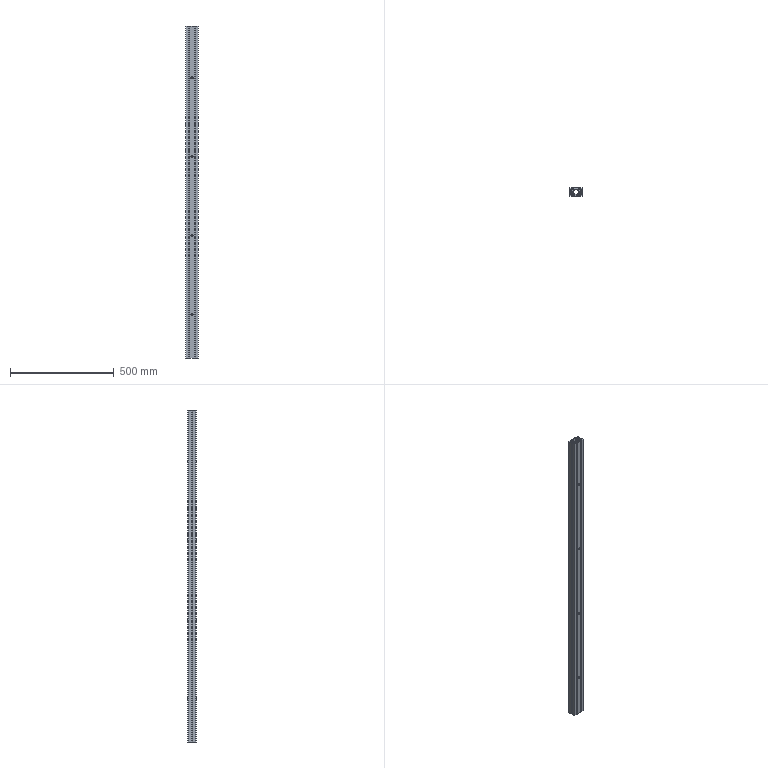Part | NX | 1 solid | 88 faces | box 60 x 40 x 1600 mm | volume 2047255 mm3 | plane 60 | cylinder 28 | commonest cylinder face diameters 10 x8 2 x4 3 x4 6 x4 19 x4 5 x2